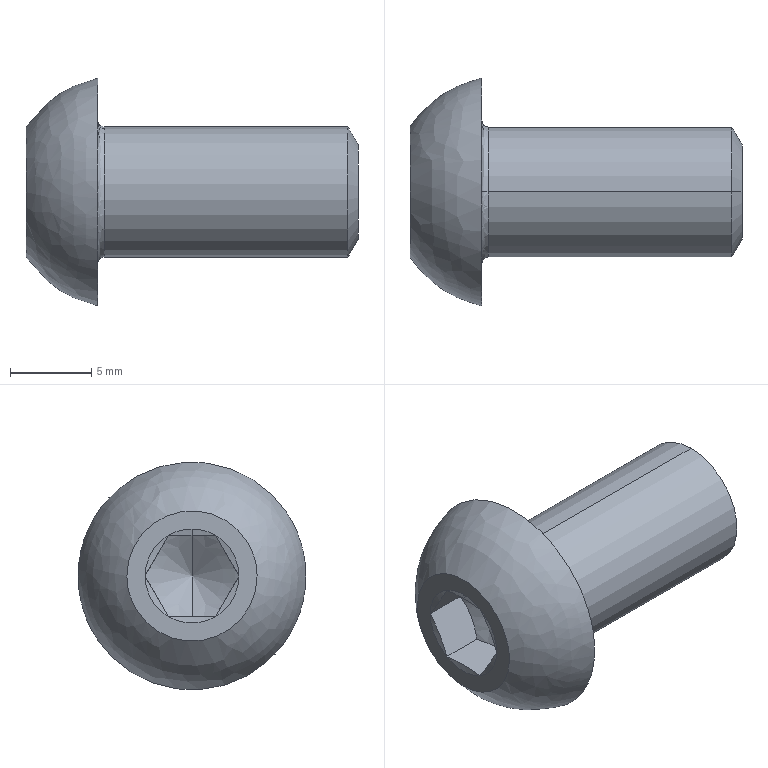Part | SolidWorks | features BaseBody 1 | 1 solid | 25 faces | box 20.4 x 14 x 14 mm | volume 1220 mm3 | cone 11 | plane 9 | spline 3 | cylinder 2 | commonest cylinder face diameters 8 x2
STEP:
#1=CARTESIAN_POINT('',(-15.6,0.,-4.));
#2=VERTEX_POINT('',#1);
#3=CARTESIAN_POINT('',(-15.6,0.,4.));
#4=VERTEX_POINT('',#3);
#5=CARTESIAN_POINT('',(-15.6,0.,0.));
#6=DIRECTION('',(1.,0.,0.));
#7=DIRECTION('',(0.,0.,1.));
#8=AXIS2_PLACEMENT_3D('',#5,#6,#7);
#9=CIRCLE('',#8,4.);
#10=EDGE_CURVE('',#2,#4,#9,.T.);
#11=ORIENTED_EDGE('',*,*,#10,.F.);
#12=CARTESIAN_POINT('',(-16.,0.,-4.4));
#13=VERTEX_POINT('',#12);
#14=CARTESIAN_POINT('',(-15.6,0.,-4.4));
#15=DIRECTION('',(0.,-1.,0.));
#16=DIRECTION('',(0.,0.,-1.));
#17=AXIS2_PLACEMENT_3D('',#14,#15,#16);
#18=CIRCLE('',#17,0.4);
#19=EDGE_CURVE('',#2,#13,#18,.T.);
#20=ORIENTED_EDGE('',*,*,#19,.T.);
#21=CARTESIAN_POINT('',(-16.,0.,4.4));
#22=VERTEX_POINT('',#21);
#23=CARTESIAN_POINT('',(-16.,0.,4.4));
#24=CARTESIAN_POINT('',(-16.,0.2798,4.4));
#25=CARTESIAN_POINT('',(-16.,0.6922,4.361));
#26=CARTESIAN_POINT('',(-16.,1.16,4.249));
#27=CARTESIAN_POINT('',(-16.,1.391,4.176));
#28=CARTESIAN_POINT('',(-16.,1.506,4.135));
#29=CARTESIAN_POINT('',(-16.,1.555,4.116));
#30=CARTESIAN_POINT('',(-16.,1.587,4.104));
#31=CARTESIAN_POINT('',(-16.,1.602,4.098));
#32=CARTESIAN_POINT('',(-16.,1.758,4.036));
#33=CARTESIAN_POINT('',(-16.,1.96,3.944));
#34=CARTESIAN_POINT('',(-16.,2.155,3.837));
#35=CARTESIAN_POINT('',(-16.,2.283,3.762));
#36=CARTESIAN_POINT('',(-16.,2.344,3.724));
#37=CARTESIAN_POINT('',(-16.,2.662,3.516));
#38=CARTESIAN_POINT('',(-16.,2.896,3.326));
#39=CARTESIAN_POINT('',(-16.,3.219,3.004));
#40=CARTESIAN_POINT('',(-16.,3.371,2.835));
#41=CARTESIAN_POINT('',(-16.,3.509,2.656));
#42=CARTESIAN_POINT('',(-16.,3.598,2.533));
#43=CARTESIAN_POINT('',(-16.,3.642,2.47));
#44=CARTESIAN_POINT('',(-16.,3.764,2.283));
#45=CARTESIAN_POINT('',(-16.,3.876,2.091));
#46=CARTESIAN_POINT('',(-16.,3.99,1.858));
#47=CARTESIAN_POINT('',(-16.,4.034,1.757));
#48=CARTESIAN_POINT('',(-16.,4.063,1.688));
#49=CARTESIAN_POINT('',(-16.,4.078,1.652));
#50=CARTESIAN_POINT('',(-16.,4.297,1.099));
#51=CARTESIAN_POINT('',(-16.,4.4,0.5599));
#52=CARTESIAN_POINT('',(-16.,4.4,-0.2799));
#53=CARTESIAN_POINT('',(-16.,4.361,-0.6923));
#54=CARTESIAN_POINT('',(-16.,4.249,-1.16));
#55=CARTESIAN_POINT('',(-16.,4.176,-1.391));
#56=CARTESIAN_POINT('',(-16.,4.135,-1.506));
#57=CARTESIAN_POINT('',(-16.,4.116,-1.555));
#58=CARTESIAN_POINT('',(-16.,4.104,-1.587));
#59=CARTESIAN_POINT('',(-16.,4.098,-1.602));
#60=CARTESIAN_POINT('',(-16.,4.036,-1.758));
#61=CARTESIAN_POINT('',(-16.,3.944,-1.96));
#62=CARTESIAN_POINT('',(-16.,3.837,-2.155));
#63=CARTESIAN_POINT('',(-16.,3.762,-2.283));
#64=CARTESIAN_POINT('',(-16.,3.724,-2.344));
#65=CARTESIAN_POINT('',(-16.,3.516,-2.662));
#66=CARTESIAN_POINT('',(-16.,3.326,-2.896));
#67=CARTESIAN_POINT('',(-16.,3.004,-3.219));
#68=CARTESIAN_POINT('',(-16.,2.835,-3.371));
#69=CARTESIAN_POINT('',(-16.,2.656,-3.509));
#70=CARTESIAN_POINT('',(-16.,2.533,-3.598));
#71=CARTESIAN_POINT('',(-16.,2.47,-3.642));
#72=CARTESIAN_POINT('',(-16.,2.283,-3.764));
#73=CARTESIAN_POINT('',(-16.,2.091,-3.876));
#74=CARTESIAN_POINT('',(-16.,1.858,-3.99));
#75=CARTESIAN_POINT('',(-16.,1.757,-4.034));
#76=CARTESIAN_POINT('',(-16.,1.688,-4.063));
#77=CARTESIAN_POINT('',(-16.,1.652,-4.078));
#78=CARTESIAN_POINT('',(-16.,1.099,-4.297));
#79=CARTESIAN_POINT('',(-16.,0.5593,-4.4));
#80=CARTESIAN_POINT('',(-16.,0.,-4.4));
#81=B_SPLINE_CURVE_WITH_KNOTS('',3,(#23,#24,#25,#26,#27,#28,#29,#30,#31,#32,#33,#34,#35,#36,#37,#38,#39,#40,#41,#42,#43,#44,#45,#46,#47,#48,#49,#50,#51,#52,#53,#54,#55,#56,#57,#58,#59,#60,#61,#62,#63,#64,#65,#66,#67,#68,#69,#70,#71,#72,#73,#74,#75,#76,#77,#78,#79,#80),.UNSPECIFIED.,.F.,.F.,(4,1,1,1,1,2,2,1,2,2,2,1,2,2,1,1,2,2,2,1,1,1,1,2,2,1,2,2,2,1,2,2,1,1,2,2,4),(0.,0.0625,0.09375,0.1094,0.1172,0.1211,0.125,0.1562,0.1719,0.1875,0.25,0.2812,0.2969,0.3125,0.3437,0.3594,0.3672,0.375,0.5,0.5625,0.5937,0.6094,0.6172,0.6211,0.625,0.6562,0.6719,0.6875,0.75,0.7812,0.7969,0.8125,0.8437,0.8594,0.8672,0.875,1.),.UNSPECIFIED.);
#82=EDGE_CURVE('',#22,#13,#81,.T.);
#83=ORIENTED_EDGE('',*,*,#82,.F.);
#84=CARTESIAN_POINT('',(-15.6,0.,4.4));
#85=DIRECTION('',(0.,1.,0.));
#86=DIRECTION('',(0.,0.,1.));
#87=AXIS2_PLACEMENT_3D('',#84,#85,#86);
#88=CIRCLE('',#87,0.4);
#89=EDGE_CURVE('',#4,#22,#88,.T.);
#90=ORIENTED_EDGE('',*,*,#89,.F.);
#91=EDGE_LOOP('',(#11,#20,#83,#90));
#92=FACE_OUTER_BOUND('',#91,.T.);
#93=CARTESIAN_POINT('',(-15.6,0.,4.));
#94=CARTESIAN_POINT('',(-15.6,8.,4.));
#95=CARTESIAN_POINT('',(-15.6,8.,-4.));
#96=CARTESIAN_POINT('',(-15.6,0.,-4.));
#97=CARTESIAN_POINT('',(-15.834,0.,4.));
#98=CARTESIAN_POINT('',(-15.834,8.,4.));
#99=CARTESIAN_POINT('',(-15.834,8.,-4.));
#100=CARTESIAN_POINT('',(-15.834,0.,-4.));
#101=CARTESIAN_POINT('',(-16.,0.,4.166));
#102=CARTESIAN_POINT('',(-16.,8.331,4.166));
#103=CARTESIAN_POINT('',(-16.,8.331,-4.166));
#104=CARTESIAN_POINT('',(-16.,0.,-4.166));
#105=CARTESIAN_POINT('',(-16.,0.,4.4));
#106=CARTESIAN_POINT('',(-16.,8.8,4.4));
#107=CARTESIAN_POINT('',(-16.,8.8,-4.4));
#108=CARTESIAN_POINT('',(-16.,0.,-4.4));
#109=(BOUNDED_SURFACE()B_SPLINE_SURFACE(3,3,((#93,#94,#95,#96),(#97,#98,#99,#100),(#101,#102,#103,#104),(#105,#106,#107,#108)),.UNSPECIFIED.,.F.,.F.,.F.)B_SPLINE_SURFACE_WITH_KNOTS((4,4),(4,4),(0.,1.),(0.,1.),.UNSPECIFIED.)GEOMETRIC_REPRESENTATION_ITEM()RATIONAL_B_SPLINE_SURFACE(((1.,0.3333,0.3333,1.),(0.8047,0.2682,0.2682,0.8047),(0.8047,0.2682,0.2682,0.8047),(1.,0.3333,0.3333,1.)))REPRESENTATION_ITEM('')SURFACE());
#110=ADVANCED_FACE('',(#92),#109,.F.);
#111=CARTESIAN_POINT('',(-0.625,0.,4.));
#112=VERTEX_POINT('',#111);
#113=CARTESIAN_POINT('',(-0.625,0.,-4.));
#114=VERTEX_POINT('',#113);
#115=CARTESIAN_POINT('',(-0.625,0.,0.));
#116=DIRECTION('',(-1.,0.,0.));
#117=DIRECTION('',(0.,0.,1.));
#118=AXIS2_PLACEMENT_3D('',#115,#116,#117);
#119=CIRCLE('',#118,4.);
#120=EDGE_CURVE('',#112,#114,#119,.T.);
#121=ORIENTED_EDGE('',*,*,#120,.T.);
#122=CARTESIAN_POINT('',(-20.4,0.,-4.));
#123=DIRECTION('',(-1.,0.,0.));
#124=VECTOR('',#123,1000.);
#125=LINE('',#122,#124);
#126=EDGE_CURVE('',#114,#2,#125,.T.);
#127=ORIENTED_EDGE('',*,*,#126,.T.);
#128=ORIENTED_EDGE('',*,*,#10,.T.);
#129=CARTESIAN_POINT('',(-20.4,0.,4.));
#130=DIRECTION('',(-1.,0.,0.));
#131=VECTOR('',#130,1000.);
#132=LINE('',#129,#131);
#133=EDGE_CURVE('',#112,#4,#132,.T.);
#134=ORIENTED_EDGE('',*,*,#133,.F.);
#135=EDGE_LOOP('',(#121,#127,#128,#134));
#136=FACE_OUTER_BOUND('',#135,.T.);
#137=CARTESIAN_POINT('',(-20.4,0.,0.));
#138=DIRECTION('',(-1.,0.,0.));
#139=DIRECTION('',(0.,0.,1.));
#140=AXIS2_PLACEMENT_3D('',#137,#138,#139);
#141=CYLINDRICAL_SURFACE('',#140,4.);
#142=ADVANCED_FACE('',(#136),#141,.T.);
#143=CARTESIAN_POINT('',(0.,0.,2.917));
#144=VERTEX_POINT('',#143);
#145=CARTESIAN_POINT('',(0.,0.,-2.917));
#146=VERTEX_POINT('',#145);
#147=CARTESIAN_POINT('',(0.,0.,0.));
#148=DIRECTION('',(-1.,0.,0.));
#149=DIRECTION('',(0.,0.,1.));
#150=AXIS2_PLACEMENT_3D('',#147,#148,#149);
#151=CIRCLE('',#150,2.917);
#152=EDGE_CURVE('',#144,#146,#151,.T.);
#153=ORIENTED_EDGE('',*,*,#152,.T.);
#154=CARTESIAN_POINT('',(-0.625,0.,-4.));
#155=DIRECTION('',(-0.5,0.,-0.866));
#156=VECTOR('',#155,1000.);
#157=LINE('',#154,#156);
#158=EDGE_CURVE('',#146,#114,#157,.T.);
#159=ORIENTED_EDGE('',*,*,#158,.T.);
#160=ORIENTED_EDGE('',*,*,#120,.F.);
#161=CARTESIAN_POINT('',(-0.625,0.,4.));
#162=DIRECTION('',(-0.5,0.,0.866));
#163=VECTOR('',#162,1000.);
#164=LINE('',#161,#163);
#165=EDGE_CURVE('',#144,#112,#164,.T.);
#166=ORIENTED_EDGE('',*,*,#165,.F.);
#167=EDGE_LOOP('',(#153,#159,#160,#166));
#168=FACE_OUTER_BOUND('',#167,.T.);
#169=CARTESIAN_POINT('',(-0.625,0.,0.));
#170=DIRECTION('',(-1.,0.,0.));
#171=DIRECTION('',(0.,0.,1.));
#172=AXIS2_PLACEMENT_3D('',#169,#170,#171);
#173=CONICAL_SURFACE('',#172,4.,1.047);
#174=ADVANCED_FACE('',(#168),#173,.T.);
#175=CARTESIAN_POINT('',(-20.4,1.443,2.5));
#176=VERTEX_POINT('',#175);
#177=CARTESIAN_POINT('',(-20.304,0.,2.5));
#178=VERTEX_POINT('',#177);
#179=CARTESIAN_POINT('',(-20.4,1.443,2.5));
#180=CARTESIAN_POINT('',(-20.34,0.9641,2.5));
#181=CARTESIAN_POINT('',(-20.304,0.4833,2.5));
#182=CARTESIAN_POINT('',(-20.304,0.,2.5));
#183=B_SPLINE_CURVE_WITH_KNOTS('',3,(#179,#180,#181,#182),.UNSPECIFIED.,.F.,.F.,(4,4),(0.,0.001447),.UNSPECIFIED.);
#184=EDGE_CURVE('',#176,#178,#183,.T.);
#185=ORIENTED_EDGE('',*,*,#184,.T.);
#186=CARTESIAN_POINT('',(-20.4,0.,2.887));
#187=VERTEX_POINT('',#186);
#188=CARTESIAN_POINT('',(-20.4,0.,2.887));
#189=DIRECTION('',(-0.242,0.,0.9703));
#190=VECTOR('',#189,1000.);
#191=LINE('',#188,#190);
#192=EDGE_CURVE('',#178,#187,#191,.T.);
#193=ORIENTED_EDGE('',*,*,#192,.T.);
#194=CARTESIAN_POINT('',(-20.4,0.,0.));
#195=DIRECTION('',(-1.,0.,0.));
#196=DIRECTION('',(0.,0.,1.));
#197=AXIS2_PLACEMENT_3D('',#194,#195,#196);
#198=CIRCLE('',#197,2.887);
#199=EDGE_CURVE('',#187,#176,#198,.T.);
#200=ORIENTED_EDGE('',*,*,#199,.T.);
#201=EDGE_LOOP('',(#185,#193,#200));
#202=FACE_OUTER_BOUND('',#201,.T.);
#203=CARTESIAN_POINT('',(-20.4,0.,0.));
#204=DIRECTION('',(-1.,0.,0.));
#205=DIRECTION('',(0.,0.,1.));
#206=AXIS2_PLACEMENT_3D('',#203,#204,#205);
#207=CONICAL_SURFACE('',#206,2.887,1.326);
#208=ADVANCED_FACE('',(#202),#207,.F.);
#209=CARTESIAN_POINT('',(-16.,0.,0.));
#210=VERTEX_POINT('',#209);
#211=CARTESIAN_POINT('',(-17.559,0.,2.5));
#212=VERTEX_POINT('',#211);
#213=CARTESIAN_POINT('',(-17.811,0.,2.904));
#214=DIRECTION('',(-0.5291,0.,0.8486));
#215=VECTOR('',#214,1000.);
#216=LINE('',#213,#215);
#217=EDGE_CURVE('',#210,#212,#216,.T.);
#218=ORIENTED_EDGE('',*,*,#217,.F.);
#219=CARTESIAN_POINT('',(-17.559,0.,-2.5));
#220=VERTEX_POINT('',#219);
#221=CARTESIAN_POINT('',(-17.811,0.,-2.904));
#222=DIRECTION('',(-0.5291,0.,-0.8486));
#223=VECTOR('',#222,1000.);
#224=LINE('',#221,#223);
#225=EDGE_CURVE('',#210,#220,#224,.T.);
#226=ORIENTED_EDGE('',*,*,#225,.T.);
#227=CARTESIAN_POINT('',(-17.8,-1.443,-2.5));
#228=VERTEX_POINT('',#227);
#229=CARTESIAN_POINT('',(-17.559,0.,-2.5));
#230=CARTESIAN_POINT('',(-17.559,-0.4946,-2.5));
#231=CARTESIAN_POINT('',(-17.653,-0.9733,-2.5));
#232=CARTESIAN_POINT('',(-17.8,-1.443,-2.5));
#233=B_SPLINE_CURVE_WITH_KNOTS('',3,(#229,#230,#231,#232),.UNSPECIFIED.,.F.,.F.,(4,4),(0.,0.001463),.UNSPECIFIED.);
#234=EDGE_CURVE('',#220,#228,#233,.T.);
#235=ORIENTED_EDGE('',*,*,#234,.T.);
#236=CARTESIAN_POINT('',(-17.8,-2.887,0.));
#237=VERTEX_POINT('',#236);
#238=CARTESIAN_POINT('',(-17.8,-1.443,-2.5));
#239=CARTESIAN_POINT('',(-17.654,-1.678,-2.093));
#240=CARTESIAN_POINT('',(-17.559,-1.917,-1.679));
#241=CARTESIAN_POINT('',(-17.559,-2.286,-1.04));
#242=CARTESIAN_POINT('',(-17.582,-2.409,-0.8268));
#243=CARTESIAN_POINT('',(-17.666,-2.65,-0.4095));
#244=CARTESIAN_POINT('',(-17.727,-2.769,-0.2038));
#245=CARTESIAN_POINT('',(-17.8,-2.887,0.));
#246=B_SPLINE_CURVE_WITH_KNOTS('',3,(#238,#239,#240,#241,#242,#243,#244,#245),.UNSPECIFIED.,.F.,.F.,(4,2,2,4),(0.,0.00146,0.002189,0.002919),.UNSPECIFIED.);
#247=EDGE_CURVE('',#228,#237,#246,.T.);
#248=ORIENTED_EDGE('',*,*,#247,.T.);
#249=CARTESIAN_POINT('',(-17.8,-1.443,2.5));
#250=VERTEX_POINT('',#249);
#251=CARTESIAN_POINT('',(-17.8,-2.887,0.));
#252=CARTESIAN_POINT('',(-17.654,-2.652,0.4068));
#253=CARTESIAN_POINT('',(-17.559,-2.413,0.8206));
#254=CARTESIAN_POINT('',(-17.559,-2.044,1.46));
#255=CARTESIAN_POINT('',(-17.582,-1.921,1.673));
#256=CARTESIAN_POINT('',(-17.666,-1.68,2.09));
#257=CARTESIAN_POINT('',(-17.727,-1.561,2.296));
#258=CARTESIAN_POINT('',(-17.8,-1.443,2.5));
#259=B_SPLINE_CURVE_WITH_KNOTS('',3,(#251,#252,#253,#254,#255,#256,#257,#258),.UNSPECIFIED.,.F.,.F.,(4,2,2,4),(0.,0.00146,0.002189,0.002919),.UNSPECIFIED.);
#260=EDGE_CURVE('',#237,#250,#259,.T.);
#261=ORIENTED_EDGE('',*,*,#260,.T.);
#262=CARTESIAN_POINT('',(-17.559,0.,2.5));
#263=CARTESIAN_POINT('',(-17.559,-0.4946,2.5));
#264=CARTESIAN_POINT('',(-17.653,-0.9733,2.5));
#265=CARTESIAN_POINT('',(-17.8,-1.443,2.5));
#266=B_SPLINE_CURVE_WITH_KNOTS('',3,(#262,#263,#264,#265),.UNSPECIFIED.,.F.,.F.,(4,4),(0.,0.001463),.UNSPECIFIED.);
#267=EDGE_CURVE('',#212,#250,#266,.T.);
#268=ORIENTED_EDGE('',*,*,#267,.F.);
#269=EDGE_LOOP('',(#218,#226,#235,#248,#261,#268));
#270=FACE_OUTER_BOUND('',#269,.T.);
#271=CARTESIAN_POINT('',(-17.811,0.,0.));
#272=DIRECTION('',(-1.,0.,0.));
#273=DIRECTION('',(0.,0.,1.));
#274=AXIS2_PLACEMENT_3D('',#271,#272,#273);
#275=CONICAL_SURFACE('',#274,2.904,1.013);
#276=ADVANCED_FACE('',(#270),#275,.F.);
#277=ORIENTED_EDGE('',*,*,#126,.F.);
#278=CARTESIAN_POINT('',(-0.625,0.,0.));
#279=DIRECTION('',(-1.,0.,0.));
#280=DIRECTION('',(0.,0.,1.));
#281=AXIS2_PLACEMENT_3D('',#278,#279,#280);
#282=CIRCLE('',#281,4.);
#283=EDGE_CURVE('',#114,#112,#282,.T.);
#284=ORIENTED_EDGE('',*,*,#283,.T.);
#285=ORIENTED_EDGE('',*,*,#133,.T.);
#286=CARTESIAN_POINT('',(-15.6,0.,0.));
#287=DIRECTION('',(1.,0.,0.));
#288=DIRECTION('',(0.,0.,1.));
#289=AXIS2_PLACEMENT_3D('',#286,#287,#288);
#290=CIRCLE('',#289,4.);
#291=EDGE_CURVE('',#4,#2,#290,.T.);
#292=ORIENTED_EDGE('',*,*,#291,.T.);
#293=EDGE_LOOP('',(#277,#284,#285,#292));
#294=FACE_OUTER_BOUND('',#293,.T.);
#295=CARTESIAN_POINT('',(-20.4,0.,0.));
#296=DIRECTION('',(-1.,0.,0.));
#297=DIRECTION('',(0.,0.,1.));
#298=AXIS2_PLACEMENT_3D('',#295,#296,#297);
#299=CYLINDRICAL_SURFACE('',#298,4.);
#300=ADVANCED_FACE('',(#294),#299,.T.);
#301=ORIENTED_EDGE('',*,*,#19,.F.);
#302=ORIENTED_EDGE('',*,*,#291,.F.);
#303=ORIENTED_EDGE('',*,*,#89,.T.);
#304=CARTESIAN_POINT('',(-16.,0.,-4.4));
#305=CARTESIAN_POINT('',(-16.,-0.2798,-4.4));
#306=CARTESIAN_POINT('',(-16.,-0.6922,-4.361));
#307=CARTESIAN_POINT('',(-16.,-1.16,-4.249));
#308=CARTESIAN_POINT('',(-16.,-1.391,-4.176));
#309=CARTESIAN_POINT('',(-16.,-1.506,-4.135));
#310=CARTESIAN_POINT('',(-16.,-1.555,-4.116));
#311=CARTESIAN_POINT('',(-16.,-1.587,-4.104));
#312=CARTESIAN_POINT('',(-16.,-1.602,-4.098));
#313=CARTESIAN_POINT('',(-16.,-1.758,-4.036));
#314=CARTESIAN_POINT('',(-16.,-1.96,-3.944));
#315=CARTESIAN_POINT('',(-16.,-2.155,-3.837));
#316=CARTESIAN_POINT('',(-16.,-2.283,-3.762));
#317=CARTESIAN_POINT('',(-16.,-2.344,-3.724));
#318=CARTESIAN_POINT('',(-16.,-2.662,-3.516));
#319=CARTESIAN_POINT('',(-16.,-2.896,-3.326));
#320=CARTESIAN_POINT('',(-16.,-3.219,-3.004));
#321=CARTESIAN_POINT('',(-16.,-3.371,-2.835));
#322=CARTESIAN_POINT('',(-16.,-3.509,-2.656));
#323=CARTESIAN_POINT('',(-16.,-3.598,-2.533));
#324=CARTESIAN_POINT('',(-16.,-3.642,-2.47));
#325=CARTESIAN_POINT('',(-16.,-3.764,-2.283));
#326=CARTESIAN_POINT('',(-16.,-3.876,-2.091));
#327=CARTESIAN_POINT('',(-16.,-3.99,-1.858));
#328=CARTESIAN_POINT('',(-16.,-4.034,-1.757));
#329=CARTESIAN_POINT('',(-16.,-4.063,-1.688));
#330=CARTESIAN_POINT('',(-16.,-4.078,-1.652));
#331=CARTESIAN_POINT('',(-16.,-4.297,-1.099));
#332=CARTESIAN_POINT('',(-16.,-4.4,-0.5599));
#333=CARTESIAN_POINT('',(-16.,-4.4,0.2799));
#334=CARTESIAN_POINT('',(-16.,-4.361,0.6923));
#335=CARTESIAN_POINT('',(-16.,-4.249,1.16));
#336=CARTESIAN_POINT('',(-16.,-4.176,1.391));
#337=CARTESIAN_POINT('',(-16.,-4.135,1.506));
#338=CARTESIAN_POINT('',(-16.,-4.116,1.555));
#339=CARTESIAN_POINT('',(-16.,-4.104,1.587));
#340=CARTESIAN_POINT('',(-16.,-4.098,1.602));
#341=CARTESIAN_POINT('',(-16.,-4.036,1.758));
#342=CARTESIAN_POINT('',(-16.,-3.944,1.96));
#343=CARTESIAN_POINT('',(-16.,-3.837,2.155));
#344=CARTESIAN_POINT('',(-16.,-3.762,2.283));
#345=CARTESIAN_POINT('',(-16.,-3.724,2.344));
#346=CARTESIAN_POINT('',(-16.,-3.516,2.662));
#347=CARTESIAN_POINT('',(-16.,-3.326,2.896));
#348=CARTESIAN_POINT('',(-16.,-3.004,3.219));
#349=CARTESIAN_POINT('',(-16.,-2.835,3.371));
#350=CARTESIAN_POINT('',(-16.,-2.656,3.509));
#351=CARTESIAN_POINT('',(-16.,-2.533,3.598));
#352=CARTESIAN_POINT('',(-16.,-2.47,3.642));
#353=CARTESIAN_POINT('',(-16.,-2.283,3.764));
#354=CARTESIAN_POINT('',(-16.,-2.091,3.876));
#355=CARTESIAN_POINT('',(-16.,-1.858,3.99));
#356=CARTESIAN_POINT('',(-16.,-1.757,4.034));
#357=CARTESIAN_POINT('',(-16.,-1.688,4.063));
#358=CARTESIAN_POINT('',(-16.,-1.652,4.078));
#359=CARTESIAN_POINT('',(-16.,-1.099,4.297));
#360=CARTESIAN_POINT('',(-16.,-0.5593,4.4));
#361=CARTESIAN_POINT('',(-16.,0.,4.4));
#362=B_SPLINE_CURVE_WITH_KNOTS('',3,(#304,#305,#306,#307,#308,#309,#310,#311,#312,#313,#314,#315,#316,#317,#318,#319,#320,#321,#322,#323,#324,#325,#326,#327,#328,#329,#330,#331,#332,#333,#334,#335,#336,#337,#338,#339,#340,#341,#342,#343,#344,#345,#346,#347,#348,#349,#350,#351,#352,#353,#354,#355,#356,#357,#358,#359,#360,#361),.UNSPECIFIED.,.F.,.F.,(4,1,1,1,1,2,2,1,2,2,2,1,2,2,1,1,2,2,2,1,1,1,1,2,2,1,2,2,2,1,2,2,1,1,2,2,4),(0.,0.0625,0.09375,0.1094,0.1172,0.1211,0.125,0.1563,0.1719,0.1875,0.25,0.2813,0.2969,0.3125,0.3438,0.3594,0.3672,0.375,0.5,0.5625,0.5938,0.6094,0.6172,0.6211,0.625,0.6563,0.6719,0.6875,0.75,0.7813,0.7969,0.8125,0.8438,0.8594,0.8672,0.875,1.),.UNSPECIFIED.);
#363=EDGE_CURVE('',#13,#22,#362,.T.);
#364=ORIENTED_EDGE('',*,*,#363,.F.);
#365=EDGE_LOOP('',(#301,#302,#303,#364));
#366=FACE_OUTER_BOUND('',#365,.T.);
#367=CARTESIAN_POINT('',(-15.6,0.,-4.));
#368=CARTESIAN_POINT('',(-15.6,-8.,-4.));
#369=CARTESIAN_POINT('',(-15.6,-8.,4.));
#370=CARTESIAN_POINT('',(-15.6,0.,4.));
#371=CARTESIAN_POINT('',(-15.834,0.,-4.));
#372=CARTESIAN_POINT('',(-15.834,-8.,-4.));
#373=CARTESIAN_POINT('',(-15.834,-8.,4.));
#374=CARTESIAN_POINT('',(-15.834,0.,4.));
#375=CARTESIAN_POINT('',(-16.,0.,-4.166));
#376=CARTESIAN_POINT('',(-16.,-8.331,-4.166));
#377=CARTESIAN_POINT('',(-16.,-8.331,4.166));
#378=CARTESIAN_POINT('',(-16.,0.,4.166));
#379=CARTESIAN_POINT('',(-16.,0.,-4.4));
#380=CARTESIAN_POINT('',(-16.,-8.8,-4.4));
#381=CARTESIAN_POINT('',(-16.,-8.8,4.4));
#382=CARTESIAN_POINT('',(-16.,0.,4.4));
#383=(BOUNDED_SURFACE()B_SPLINE_SURFACE(3,3,((#367,#368,#369,#370),(#371,#372,#373,#374),(#375,#376,#377,#378),(#379,#380,#381,#382)),.UNSPECIFIED.,.F.,.F.,.F.)B_SPLINE_SURFACE_WITH_KNOTS((4,4),(4,4),(0.,1.),(0.,1.),.UNSPECIFIED.)GEOMETRIC_REPRESENTATION_ITEM()RATIONAL_B_SPLINE_SURFACE(((1.,0.3333,0.3333,1.),(0.8047,0.2682,0.2682,0.8047),(0.8047,0.2682,0.2682,0.8047),(1.,0.3333,0.3333,1.)))REPRESENTATION_ITEM('')SURFACE());
#384=ADVANCED_FACE('',(#366),#383,.F.);
#385=ORIENTED_EDGE('',*,*,#158,.F.);
#386=CARTESIAN_POINT('',(0.,0.,0.));
#387=DIRECTION('',(-1.,0.,0.));
#388=DIRECTION('',(0.,0.,1.));
#389=AXIS2_PLACEMENT_3D('',#386,#387,#388);
#390=CIRCLE('',#389,2.917);
#391=EDGE_CURVE('',#146,#144,#390,.T.);
#392=ORIENTED_EDGE('',*,*,#391,.T.);
#393=ORIENTED_EDGE('',*,*,#165,.T.);
#394=ORIENTED_EDGE('',*,*,#283,.F.);
#395=EDGE_LOOP('',(#385,#392,#393,#394));
#396=FACE_OUTER_BOUND('',#395,.T.);
#397=CARTESIAN_POINT('',(-0.625,0.,0.));
#398=DIRECTION('',(-1.,0.,0.));
#399=DIRECTION('',(0.,0.,1.));
#400=AXIS2_PLACEMENT_3D('',#397,#398,#399);
#401=CONICAL_SURFACE('',#400,4.,1.047);
#402=ADVANCED_FACE('',(#396),#401,.T.);
#403=ORIENTED_EDGE('',*,*,#363,.T.);
#404=ORIENTED_EDGE('',*,*,#82,.T.);
#405=EDGE_LOOP('',(#403,#404));
#406=FACE_BOUND('',#405,.T.);
#407=CARTESIAN_POINT('',(-16.,7.,0.));
#408=VERTEX_POINT('',#407);
#409=CARTESIAN_POINT('',(-16.,-7.,0.));
#410=VERTEX_POINT('',#409);
#411=CARTESIAN_POINT('',(-16.,7.,0.));
#412=CARTESIAN_POINT('',(-16.,7.,-0.4622));
#413=CARTESIAN_POINT('',(-16.,6.955,-0.9197));
#414=CARTESIAN_POINT('',(-16.,6.774,-1.825));
#415=CARTESIAN_POINT('',(-16.,6.64,-2.263));
#416=CARTESIAN_POINT('',(-16.,6.378,-2.895));
#417=CARTESIAN_POINT('',(-16.,6.28,-3.101));
#418=CARTESIAN_POINT('',(-16.,6.063,-3.506));
#419=CARTESIAN_POINT('',(-16.,5.944,-3.704));
#420=CARTESIAN_POINT('',(-16.,5.561,-4.277));
#421=CARTESIAN_POINT('',(-16.,5.271,-4.629));
#422=CARTESIAN_POINT('',(-16.,4.625,-5.274));
#423=CARTESIAN_POINT('',(-16.,4.264,-5.57));
#424=CARTESIAN_POINT('',(-16.,3.505,-6.077));
#425=CARTESIAN_POINT('',(-16.,3.103,-6.292));
#426=CARTESIAN_POINT('',(-16.,2.466,-6.555));
#427=CARTESIAN_POINT('',(-16.,2.248,-6.633));
#428=CARTESIAN_POINT('',(-16.,1.809,-6.766));
#429=CARTESIAN_POINT('',(-16.,1.587,-6.821));
#430=CARTESIAN_POINT('',(-16.,0.917,-6.955));
#431=CARTESIAN_POINT('',(-16.,0.4599,-7.));
#432=CARTESIAN_POINT('',(-16.,-0.4622,-7.));
#433=CARTESIAN_POINT('',(-16.,-0.9163,-6.955));
#434=CARTESIAN_POINT('',(-16.,-1.587,-6.821));
#435=CARTESIAN_POINT('',(-16.,-1.809,-6.766));
#436=CARTESIAN_POINT('',(-16.,-2.25,-6.633));
#437=CARTESIAN_POINT('',(-16.,-2.468,-6.555));
#438=CARTESIAN_POINT('',(-16.,-3.102,-6.292));
#439=CARTESIAN_POINT('',(-16.,-3.504,-6.077));
#440=CARTESIAN_POINT('',(-16.,-4.075,-5.696));
#441=CARTESIAN_POINT('',(-16.,-4.261,-5.558));
#442=CARTESIAN_POINT('',(-16.,-4.617,-5.266));
#443=CARTESIAN_POINT('',(-16.,-4.787,-5.113));
#444=CARTESIAN_POINT('',(-16.,-5.271,-4.629));
#445=CARTESIAN_POINT('',(-16.,-5.561,-4.277));
#446=CARTESIAN_POINT('',(-16.,-6.073,-3.511));
#447=CARTESIAN_POINT('',(-16.,-6.29,-3.105));
#448=CARTESIAN_POINT('',(-16.,-6.552,-2.474));
#449=CARTESIAN_POINT('',(-16.,-6.629,-2.259));
#450=CARTESIAN_POINT('',(-16.,-6.763,-1.821));
#451=CARTESIAN_POINT('',(-16.,-6.819,-1.596));
#452=CARTESIAN_POINT('',(-16.,-6.955,-0.919));
#453=CARTESIAN_POINT('',(-16.,-7.,-0.4622));
#454=CARTESIAN_POINT('',(-16.,-7.,0.));
#455=B_SPLINE_CURVE_WITH_KNOTS('',3,(#411,#412,#413,#414,#415,#416,#417,#418,#419,#420,#421,#422,#423,#424,#425,#426,#427,#428,#429,#430,#431,#432,#433,#434,#435,#436,#437,#438,#439,#440,#441,#442,#443,#444,#445,#446,#447,#448,#449,#450,#451,#452,#453,#454),.UNSPECIFIED.,.F.,.F.,(4,2,2,2,2,2,2,2,2,2,2,2,2,2,2,2,2,2,2,2,2,4),(0.,0.001379,0.002758,0.003448,0.004138,0.005517,0.006896,0.008275,0.008965,0.009654,0.01103,0.01241,0.0131,0.01379,0.01517,0.01586,0.01655,0.01793,0.01931,0.02,0.02069,0.02207),.UNSPECIFIED.);
#456=EDGE_CURVE('',#408,#410,#455,.T.);
#457=ORIENTED_EDGE('',*,*,#456,.F.);
#458=CARTESIAN_POINT('',(-16.,-7.,0.));
#459=CARTESIAN_POINT('',(-16.,-7.,0.4622));
#460=CARTESIAN_POINT('',(-16.,-6.955,0.9197));
#461=CARTESIAN_POINT('',(-16.,-6.774,1.825));
#462=CARTESIAN_POINT('',(-16.,-6.64,2.263));
#463=CARTESIAN_POINT('',(-16.,-6.378,2.895));
#464=CARTESIAN_POINT('',(-16.,-6.28,3.101));
#465=CARTESIAN_POINT('',(-16.,-6.063,3.506));
#466=CARTESIAN_POINT('',(-16.,-5.944,3.704));
#467=CARTESIAN_POINT('',(-16.,-5.561,4.277));
#468=CARTESIAN_POINT('',(-16.,-5.271,4.629));
#469=CARTESIAN_POINT('',(-16.,-4.625,5.274));
#470=CARTESIAN_POINT('',(-16.,-4.264,5.57));
#471=CARTESIAN_POINT('',(-16.,-3.505,6.077));
#472=CARTESIAN_POINT('',(-16.,-3.103,6.292));
#473=CARTESIAN_POINT('',(-16.,-2.466,6.555));
#474=CARTESIAN_POINT('',(-16.,-2.248,6.633));
#475=CARTESIAN_POINT('',(-16.,-1.809,6.766));
#476=CARTESIAN_POINT('',(-16.,-1.587,6.821));
#477=CARTESIAN_POINT('',(-16.,-0.917,6.955));
#478=CARTESIAN_POINT('',(-16.,-0.4599,7.));
#479=CARTESIAN_POINT('',(-16.,0.4622,7.));
#480=CARTESIAN_POINT('',(-16.,0.9163,6.955));
#481=CARTESIAN_POINT('',(-16.,1.587,6.821));
#482=CARTESIAN_POINT('',(-16.,1.809,6.766));
#483=CARTESIAN_POINT('',(-16.,2.25,6.633));
#484=CARTESIAN_POINT('',(-16.,2.468,6.555));
#485=CARTESIAN_POINT('',(-16.,3.102,6.292));
#486=CARTESIAN_POINT('',(-16.,3.504,6.077));
#487=CARTESIAN_POINT('',(-16.,4.075,5.696));
#488=CARTESIAN_POINT('',(-16.,4.261,5.558));
#489=CARTESIAN_POINT('',(-16.,4.617,5.266));
#490=CARTESIAN_POINT('',(-16.,4.787,5.113));
#491=CARTESIAN_POINT('',(-16.,5.271,4.629));
#492=CARTESIAN_POINT('',(-16.,5.561,4.277));
#493=CARTESIAN_POINT('',(-16.,6.073,3.511));
#494=CARTESIAN_POINT('',(-16.,6.29,3.105));
#495=CARTESIAN_POINT('',(-16.,6.552,2.474));
#496=CARTESIAN_POINT('',(-16.,6.629,2.259));
#497=CARTESIAN_POINT('',(-16.,6.763,1.821));
#498=CARTESIAN_POINT('',(-16.,6.819,1.596));
#499=CARTESIAN_POINT('',(-16.,6.955,0.919));
#500=CARTESIAN_POINT('',(-16.,7.,0.4622));
#501=CARTESIAN_POINT('',(-16.,7.,0.));
#502=B_SPLINE_CURVE_WITH_KNOTS('',3,(#458,#459,#460,#461,#462,#463,#464,#465,#466,#467,#468,#469,#470,#471,#472,#473,#474,#475,#476,#477,#478,#479,#480,#481,#482,#483,#484,#485,#486,#487,#488,#489,#490,#491,#492,#493,#494,#495,#496,#497,#498,#499,#500,#501),.UNSPECIFIED.,.F.,.F.,(4,2,2,2,2,2,2,2,2,2,2,2,2,2,2,2,2,2,2,2,2,4),(0.02207,0.02345,0.02483,0.02552,0.0262,0.02758,0.02896,0.03034,0.03103,0.03172,0.0331,0.03448,0.03517,0.03586,0.03724,0.03793,0.03862,0.04,0.04138,0.04207,0.04276,0.04413),.UNSPECIFIED.);
#503=EDGE_CURVE('',#410,#408,#502,.T.);
#504=ORIENTED_EDGE('',*,*,#503,.F.);
#505=EDGE_LOOP('',(#457,#504));
#506=FACE_OUTER_BOUND('',#505,.T.);
#507=CARTESIAN_POINT('',(-16.,4.4,0.));
#508=DIRECTION('',(-1.,0.,0.));
#509=DIRECTION('',(0.,0.,1.));
#510=AXIS2_PLACEMENT_3D('',#507,#508,#509);
#511=PLANE('',#510);
#512=ADVANCED_FACE('',(#406,#506),#511,.F.);
#513=ORIENTED_EDGE('',*,*,#152,.F.);
#514=ORIENTED_EDGE('',*,*,#391,.F.);
#515=EDGE_LOOP('',(#513,#514));
#516=FACE_OUTER_BOUND('',#515,.T.);
#517=CARTESIAN_POINT('',(0.,4.,0.));
#518=DIRECTION('',(-1.,0.,0.));
#519=DIRECTION('',(0.,0.,1.));
#520=AXIS2_PLACEMENT_3D('',#517,#518,#519);
#521=PLANE('',#520);
#522=ADVANCED_FACE('',(#516),#521,.F.);
#523=CARTESIAN_POINT('',(-20.4,-4.,0.));
#524=VERTEX_POINT('',#523);
#525=CARTESIAN_POINT('',(-20.4,4.,0.));
#526=VERTEX_POINT('',#525);
#527=CARTESIAN_POINT('',(-20.4,-4.,0.));
#528=CARTESIAN_POINT('',(-20.4,-4.,-0.2642));
#529=CARTESIAN_POINT('',(-20.4,-3.974,-0.5241));
#530=CARTESIAN_POINT('',(-20.4,-3.872,-1.035));
#531=CARTESIAN_POINT('',(-20.4,-3.796,-1.289));
#532=CARTESIAN_POINT('',(-20.4,-3.595,-1.774));
#533=CARTESIAN_POINT('',(-20.4,-3.472,-2.003));
#534=CARTESIAN_POINT('',(-20.4,-3.182,-2.438));
#535=CARTESIAN_POINT('',(-20.4,-3.013,-2.644));
#536=CARTESIAN_POINT('',(-20.4,-2.644,-3.013));
#537=CARTESIAN_POINT('',(-20.4,-2.443,-3.179));
#538=CARTESIAN_POINT('',(-20.4,-2.005,-3.471));
#539=CARTESIAN_POINT('',(-20.4,-1.773,-3.595));
#540=CARTESIAN_POINT('',(-20.4,-1.291,-3.795));
#541=CARTESIAN_POINT('',(-20.4,-1.039,-3.872));
#542=CARTESIAN_POINT('',(-20.4,-0.523,-3.974));
#543=CARTESIAN_POINT('',(-20.4,-0.2635,-4.));
#544=CARTESIAN_POINT('',(-20.4,0.2581,-4.));
#545=CARTESIAN_POINT('',(-20.4,0.5231,-3.974));
#546=CARTESIAN_POINT('',(-20.4,1.036,-3.872));
#547=CARTESIAN_POINT('',(-20.4,1.285,-3.797));
#548=CARTESIAN_POINT('',(-20.4,1.77,-3.597));
#549=CARTESIAN_POINT('',(-20.4,2.004,-3.472));
#550=CARTESIAN_POINT('',(-20.4,2.437,-3.182));
#551=CARTESIAN_POINT('',(-20.4,2.64,-3.017));
#552=CARTESIAN_POINT('',(-20.4,3.013,-2.644));
#553=CARTESIAN_POINT('',(-20.4,3.179,-2.442));
#554=CARTESIAN_POINT('',(-20.4,3.469,-2.009));
#555=CARTESIAN_POINT('',(-20.4,3.594,-1.775));
#556=CARTESIAN_POINT('',(-20.4,3.795,-1.29));
#557=CARTESIAN_POINT('',(-20.4,3.871,-1.041));
#558=CARTESIAN_POINT('',(-20.4,3.974,-0.5286));
#559=CARTESIAN_POINT('',(-20.4,4.,-0.2642));
#560=CARTESIAN_POINT('',(-20.4,4.,0.));
#561=B_SPLINE_CURVE_WITH_KNOTS('',3,(#527,#528,#529,#530,#531,#532,#533,#534,#535,#536,#537,#538,#539,#540,#541,#542,#543,#544,#545,#546,#547,#548,#549,#550,#551,#552,#553,#554,#555,#556,#557,#558,#559,#560),.UNSPECIFIED.,.F.,.F.,(4,2,2,2,2,2,2,2,2,2,2,2,2,2,2,2,4),(0.,0.0007815,0.001563,0.002344,0.003126,0.003907,0.004689,0.00547,0.006252,0.007033,0.007815,0.008596,0.009377,0.01016,0.01094,0.01172,0.0125),.UNSPECIFIED.);
#562=EDGE_CURVE('',#524,#526,#561,.T.);
#563=ORIENTED_EDGE('',*,*,#562,.T.);
#564=CARTESIAN_POINT('',(-20.4,4.,0.));
#565=CARTESIAN_POINT('',(-20.4,4.,0.2642));
#566=CARTESIAN_POINT('',(-20.4,3.974,0.5241));
#567=CARTESIAN_POINT('',(-20.4,3.872,1.035));
#568=CARTESIAN_POINT('',(-20.4,3.796,1.289));
#569=CARTESIAN_POINT('',(-20.4,3.595,1.774));
#570=CARTESIAN_POINT('',(-20.4,3.472,2.003));
#571=CARTESIAN_POINT('',(-20.4,3.182,2.438));
#572=CARTESIAN_POINT('',(-20.4,3.013,2.644));
#573=CARTESIAN_POINT('',(-20.4,2.644,3.013));
#574=CARTESIAN_POINT('',(-20.4,2.443,3.179));
#575=CARTESIAN_POINT('',(-20.4,2.005,3.471));
#576=CARTESIAN_POINT('',(-20.4,1.773,3.595));
#577=CARTESIAN_POINT('',(-20.4,1.291,3.795));
#578=CARTESIAN_POINT('',(-20.4,1.039,3.872));
#579=CARTESIAN_POINT('',(-20.4,0.523,3.974));
#580=CARTESIAN_POINT('',(-20.4,0.2635,4.));
#581=CARTESIAN_POINT('',(-20.4,-0.2581,4.));
#582=CARTESIAN_POINT('',(-20.4,-0.5231,3.974));
#583=CARTESIAN_POINT('',(-20.4,-1.036,3.872));
#584=CARTESIAN_POINT('',(-20.4,-1.285,3.797));
#585=CARTESIAN_POINT('',(-20.4,-1.77,3.597));
#586=CARTESIAN_POINT('',(-20.4,-2.004,3.472));
#587=CARTESIAN_POINT('',(-20.4,-2.437,3.182));
#588=CARTESIAN_POINT('',(-20.4,-2.64,3.017));
#589=CARTESIAN_POINT('',(-20.4,-3.013,2.644));
#590=CARTESIAN_POINT('',(-20.4,-3.179,2.442));
#591=CARTESIAN_POINT('',(-20.4,-3.469,2.009));
#592=CARTESIAN_POINT('',(-20.4,-3.594,1.775));
#593=CARTESIAN_POINT('',(-20.4,-3.795,1.29));
#594=CARTESIAN_POINT('',(-20.4,-3.871,1.041));
#595=CARTESIAN_POINT('',(-20.4,-3.974,0.5286));
#596=CARTESIAN_POINT('',(-20.4,-4.,0.2642));
#597=CARTESIAN_POINT('',(-20.4,-4.,0.));
#598=B_SPLINE_CURVE_WITH_KNOTS('',3,(#564,#565,#566,#567,#568,#569,#570,#571,#572,#573,#574,#575,#576,#577,#578,#579,#580,#581,#582,#583,#584,#585,#586,#587,#588,#589,#590,#591,#592,#593,#594,#595,#596,#597),.UNSPECIFIED.,.F.,.F.,(4,2,2,2,2,2,2,2,2,2,2,2,2,2,2,2,4),(0.0125,0.01328,0.01407,0.01485,0.01563,0.01641,0.01719,0.01797,0.01875,0.01954,0.02032,0.0211,0.02188,0.02266,0.02344,0.02423,0.02501),.UNSPECIFIED.);
#599=EDGE_CURVE('',#526,#524,#598,.T.);
#600=ORIENTED_EDGE('',*,*,#599,.T.);
#601=EDGE_LOOP('',(#563,#600));
#602=FACE_BOUND('',#601,.T.);
#603=ORIENTED_EDGE('',*,*,#456,.T.);
#604=ORIENTED_EDGE('',*,*,#503,.T.);
#605=EDGE_LOOP('',(#603,#604));
#606=FACE_OUTER_BOUND('',#605,.T.);
#607=CARTESIAN_POINT('',(-14.737,7.024,-1.407));
#608=CARTESIAN_POINT('',(-16.707,7.024,-1.005));
#609=CARTESIAN_POINT('',(-16.707,7.024,1.005));
#610=CARTESIAN_POINT('',(-14.737,7.024,1.407));
#611=CARTESIAN_POINT('',(-16.702,5.015,-11.035));
#612=CARTESIAN_POINT('',(-32.149,5.015,-7.883));
#613=CARTESIAN_POINT('',(-32.149,5.015,7.883));
#614=CARTESIAN_POINT('',(-16.702,5.015,11.035));
#615=CARTESIAN_POINT('',(-16.702,-5.015,-11.035));
#616=CARTESIAN_POINT('',(-32.149,-5.015,-7.883));
#617=CARTESIAN_POINT('',(-32.149,-5.015,7.883));
#618=CARTESIAN_POINT('',(-16.702,-5.015,11.035));
#619=CARTESIAN_POINT('',(-14.737,-7.024,-1.407));
#620=CARTESIAN_POINT('',(-16.707,-7.024,-1.005));
#621=CARTESIAN_POINT('',(-16.707,-7.024,1.005));
#622=CARTESIAN_POINT('',(-14.737,-7.024,1.407));
#623=(BOUNDED_SURFACE()B_SPLINE_SURFACE(3,3,((#607,#608,#609,#610),(#611,#612,#613,#614),(#615,#616,#617,#618),(#619,#620,#621,#622)),.UNSPECIFIED.,.F.,.F.,.F.)B_SPLINE_SURFACE_WITH_KNOTS((4,4),(4,4),(0.,1.),(0.,1.),.UNSPECIFIED.)GEOMETRIC_REPRESENTATION_ITEM()RATIONAL_B_SPLINE_SURFACE(((1.,0.4667,0.4667,1.),(0.4669,0.2179,0.2179,0.4669),(0.4669,0.2179,0.2179,0.4669),(1.,0.4667,0.4667,1.)))REPRESENTATION_ITEM('')SURFACE());
#624=ADVANCED_FACE('',(#602,#606),#623,.T.);
#625=CARTESIAN_POINT('',(-20.4,1.443,-2.5));
#626=VERTEX_POINT('',#625);
#627=CARTESIAN_POINT('',(-20.4,-1.443,-2.5));
#628=VERTEX_POINT('',#627);
#629=CARTESIAN_POINT('',(-20.4,0.,0.));
#630=DIRECTION('',(-1.,0.,0.));
#631=DIRECTION('',(0.,0.,1.));
#632=AXIS2_PLACEMENT_3D('',#629,#630,#631);
#633=CIRCLE('',#632,2.887);
#634=EDGE_CURVE('',#626,#628,#633,.T.);
#635=ORIENTED_EDGE('',*,*,#634,.F.);
#636=CARTESIAN_POINT('',(-20.4,2.887,0.));
#637=VERTEX_POINT('',#636);
#638=CARTESIAN_POINT('',(-20.4,0.,0.));
#639=DIRECTION('',(-1.,0.,0.));
#640=DIRECTION('',(0.,0.,1.));
#641=AXIS2_PLACEMENT_3D('',#638,#639,#640);
#642=CIRCLE('',#641,2.887);
#643=EDGE_CURVE('',#637,#626,#642,.T.);
#644=ORIENTED_EDGE('',*,*,#643,.F.);
#645=CARTESIAN_POINT('',(-20.4,0.,0.));
#646=DIRECTION('',(-1.,0.,0.));
#647=DIRECTION('',(0.,0.,1.));
#648=AXIS2_PLACEMENT_3D('',#645,#646,#647);
#649=CIRCLE('',#648,2.887);
#650=EDGE_CURVE('',#176,#637,#649,.T.);
#651=ORIENTED_EDGE('',*,*,#650,.F.);
#652=ORIENTED_EDGE('',*,*,#199,.F.);
#653=CARTESIAN_POINT('',(-20.4,-1.443,2.5));
#654=VERTEX_POINT('',#653);
#655=CARTESIAN_POINT('',(-20.4,0.,0.));
#656=DIRECTION('',(-1.,0.,0.));
#657=DIRECTION('',(0.,0.,1.));
#658=AXIS2_PLACEMENT_3D('',#655,#656,#657);
#659=CIRCLE('',#658,2.887);
#660=EDGE_CURVE('',#654,#187,#659,.T.);
#661=ORIENTED_EDGE('',*,*,#660,.F.);
#662=CARTESIAN_POINT('',(-20.4,-2.887,0.));
#663=VERTEX_POINT('',#662);
#664=CARTESIAN_POINT('',(-20.4,0.,0.));
#665=DIRECTION('',(-1.,0.,0.));
#666=DIRECTION('',(0.,0.,1.));
#667=AXIS2_PLACEMENT_3D('',#664,#665,#666);
#668=CIRCLE('',#667,2.887);
#669=EDGE_CURVE('',#663,#654,#668,.T.);
#670=ORIENTED_EDGE('',*,*,#669,.F.);
#671=CARTESIAN_POINT('',(-20.4,0.,0.));
#672=DIRECTION('',(-1.,0.,0.));
#673=DIRECTION('',(0.,0.,1.));
#674=AXIS2_PLACEMENT_3D('',#671,#672,#673);
#675=CIRCLE('',#674,2.887);
#676=EDGE_CURVE('',#628,#663,#675,.T.);
#677=ORIENTED_EDGE('',*,*,#676,.F.);
#678=EDGE_LOOP('',(#635,#644,#651,#652,#661,#670,#677));
#679=FACE_BOUND('',#678,.T.);
#680=ORIENTED_EDGE('',*,*,#562,.F.);
#681=ORIENTED_EDGE('',*,*,#599,.F.);
#682=EDGE_LOOP('',(#680,#681));
#683=FACE_OUTER_BOUND('',#682,.T.);
#684=CARTESIAN_POINT('',(-20.4,0.,0.));
#685=DIRECTION('',(1.,0.,0.));
#686=DIRECTION('',(0.,0.,-1.));
#687=AXIS2_PLACEMENT_3D('',#684,#685,#686);
#688=PLANE('',#687);
#689=ADVANCED_FACE('',(#679,#683),#688,.F.);
#690=ORIENTED_EDGE('',*,*,#676,.T.);
#691=CARTESIAN_POINT('',(-20.4,-1.443,-2.5));
#692=CARTESIAN_POINT('',(-20.34,-1.684,-2.083));
#693=CARTESIAN_POINT('',(-20.267,-2.165,-1.25));
#694=CARTESIAN_POINT('',(-20.34,-2.646,-0.4167));
#695=CARTESIAN_POINT('',(-20.4,-2.887,0.));
#696=B_SPLINE_CURVE_WITH_KNOTS('',3,(#691,#692,#693,#694,#695),.UNSPECIFIED.,.F.,.F.,(4,1,4),(0.,0.001443,0.002887),.UNSPECIFIED.);
#697=EDGE_CURVE('',#628,#663,#696,.T.);
#698=ORIENTED_EDGE('',*,*,#697,.F.);
#699=EDGE_LOOP('',(#690,#698));
#700=FACE_OUTER_BOUND('',#699,.T.);
#701=CARTESIAN_POINT('',(-20.4,0.,0.));
#702=DIRECTION('',(-1.,0.,0.));
#703=DIRECTION('',(0.,0.,1.));
#704=AXIS2_PLACEMENT_3D('',#701,#702,#703);
#705=CONICAL_SURFACE('',#704,2.887,1.326);
#706=ADVANCED_FACE('',(#700),#705,.F.);
#707=ORIENTED_EDGE('',*,*,#634,.T.);
#708=CARTESIAN_POINT('',(-20.4,1.443,-2.5));
#709=CARTESIAN_POINT('',(-20.34,0.9623,-2.5));
#710=CARTESIAN_POINT('',(-20.267,0.,-2.5));
#711=CARTESIAN_POINT('',(-20.34,-0.9623,-2.5));
#712=CARTESIAN_POINT('',(-20.4,-1.443,-2.5));
#713=B_SPLINE_CURVE_WITH_KNOTS('',3,(#708,#709,#710,#711,#712),.UNSPECIFIED.,.F.,.F.,(4,1,4),(0.,0.001443,0.002887),.UNSPECIFIED.);
#714=EDGE_CURVE('',#626,#628,#713,.T.);
#715=ORIENTED_EDGE('',*,*,#714,.F.);
#716=EDGE_LOOP('',(#707,#715));
#717=FACE_OUTER_BOUND('',#716,.T.);
#718=CARTESIAN_POINT('',(-20.4,0.,0.));
#719=DIRECTION('',(-1.,0.,0.));
#720=DIRECTION('',(0.,0.,1.));
#721=AXIS2_PLACEMENT_3D('',#718,#719,#720);
#722=CONICAL_SURFACE('',#721,2.887,1.326);
#723=ADVANCED_FACE('',(#717),#722,.F.);
#724=ORIENTED_EDGE('',*,*,#643,.T.);
#725=CARTESIAN_POINT('',(-20.4,2.887,0.));
#726=CARTESIAN_POINT('',(-20.34,2.646,-0.4167));
#727=CARTESIAN_POINT('',(-20.267,2.165,-1.25));
#728=CARTESIAN_POINT('',(-20.34,1.684,-2.083));
#729=CARTESIAN_POINT('',(-20.4,1.443,-2.5));
#730=B_SPLINE_CURVE_WITH_KNOTS('',3,(#725,#726,#727,#728,#729),.UNSPECIFIED.,.F.,.F.,(4,1,4),(0.,0.001443,0.002887),.UNSPECIFIED.);
#731=EDGE_CURVE('',#637,#626,#730,.T.);
#732=ORIENTED_EDGE('',*,*,#731,.F.);
#733=EDGE_LOOP('',(#724,#732));
#734=FACE_OUTER_BOUND('',#733,.T.);
#735=CARTESIAN_POINT('',(-20.4,0.,0.));
#736=DIRECTION('',(-1.,0.,0.));
#737=DIRECTION('',(0.,0.,1.));
#738=AXIS2_PLACEMENT_3D('',#735,#736,#737);
#739=CONICAL_SURFACE('',#738,2.887,1.326);
#740=ADVANCED_FACE('',(#734),#739,.F.);
#741=ORIENTED_EDGE('',*,*,#650,.T.);
#742=CARTESIAN_POINT('',(-20.4,1.443,2.5));
#743=CARTESIAN_POINT('',(-20.34,1.684,2.083));
#744=CARTESIAN_POINT('',(-20.267,2.165,1.25));
#745=CARTESIAN_POINT('',(-20.34,2.646,0.4167));
#746=CARTESIAN_POINT('',(-20.4,2.887,0.));
#747=B_SPLINE_CURVE_WITH_KNOTS('',3,(#742,#743,#744,#745,#746),.UNSPECIFIED.,.F.,.F.,(4,1,4),(0.,0.001443,0.002887),.UNSPECIFIED.);
#748=EDGE_CURVE('',#176,#637,#747,.T.);
#749=ORIENTED_EDGE('',*,*,#748,.F.);
#750=EDGE_LOOP('',(#741,#749));
#751=FACE_OUTER_BOUND('',#750,.T.);
#752=CARTESIAN_POINT('',(-20.4,0.,0.));
#753=DIRECTION('',(-1.,0.,0.));
#754=DIRECTION('',(0.,0.,1.));
#755=AXIS2_PLACEMENT_3D('',#752,#753,#754);
#756=CONICAL_SURFACE('',#755,2.887,1.326);
#757=ADVANCED_FACE('',(#751),#756,.F.);
#758=ORIENTED_EDGE('',*,*,#192,.F.);
#759=CARTESIAN_POINT('',(-20.304,0.,2.5));
#760=CARTESIAN_POINT('',(-20.304,-0.4833,2.5));
#761=CARTESIAN_POINT('',(-20.34,-0.9641,2.5));
#762=CARTESIAN_POINT('',(-20.4,-1.443,2.5));
#763=B_SPLINE_CURVE_WITH_KNOTS('',3,(#759,#760,#761,#762),.UNSPECIFIED.,.F.,.F.,(4,4),(0.001447,0.002893),.UNSPECIFIED.);
#764=EDGE_CURVE('',#178,#654,#763,.T.);
#765=ORIENTED_EDGE('',*,*,#764,.T.);
#766=ORIENTED_EDGE('',*,*,#660,.T.);
#767=EDGE_LOOP('',(#758,#765,#766));
#768=FACE_OUTER_BOUND('',#767,.T.);
#769=CARTESIAN_POINT('',(-20.4,0.,0.));
#770=DIRECTION('',(-1.,0.,0.));
#771=DIRECTION('',(0.,0.,1.));
#772=AXIS2_PLACEMENT_3D('',#769,#770,#771);
#773=CONICAL_SURFACE('',#772,2.887,1.326);
#774=ADVANCED_FACE('',(#768),#773,.F.);
#775=ORIENTED_EDGE('',*,*,#669,.T.);
#776=CARTESIAN_POINT('',(-20.4,-2.887,0.));
#777=CARTESIAN_POINT('',(-20.34,-2.646,0.4167));
#778=CARTESIAN_POINT('',(-20.267,-2.165,1.25));
#779=CARTESIAN_POINT('',(-20.34,-1.684,2.083));
#780=CARTESIAN_POINT('',(-20.4,-1.443,2.5));
#781=B_SPLINE_CURVE_WITH_KNOTS('',3,(#776,#777,#778,#779,#780),.UNSPECIFIED.,.F.,.F.,(4,1,4),(0.,0.001443,0.002887),.UNSPECIFIED.);
#782=EDGE_CURVE('',#663,#654,#781,.T.);
#783=ORIENTED_EDGE('',*,*,#782,.F.);
#784=EDGE_LOOP('',(#775,#783));
#785=FACE_OUTER_BOUND('',#784,.T.);
#786=CARTESIAN_POINT('',(-20.4,0.,0.));
#787=DIRECTION('',(-1.,0.,0.));
#788=DIRECTION('',(0.,0.,1.));
#789=AXIS2_PLACEMENT_3D('',#786,#787,#788);
#790=CONICAL_SURFACE('',#789,2.887,1.326);
#791=ADVANCED_FACE('',(#785),#790,.F.);
#792=CARTESIAN_POINT('',(-16.,-2.887,0.));
#793=DIRECTION('',(-1.,0.,0.));
#794=VECTOR('',#793,1000.);
#795=LINE('',#792,#794);
#796=EDGE_CURVE('',#237,#663,#795,.T.);
#797=ORIENTED_EDGE('',*,*,#796,.F.);
#798=ORIENTED_EDGE('',*,*,#247,.F.);
#799=CARTESIAN_POINT('',(-16.,-1.443,-2.5));
#800=DIRECTION('',(1.,0.,0.));
#801=VECTOR('',#800,1000.);
#802=LINE('',#799,#801);
#803=EDGE_CURVE('',#628,#228,#802,.T.);
#804=ORIENTED_EDGE('',*,*,#803,.F.);
#805=ORIENTED_EDGE('',*,*,#697,.T.);
#806=EDGE_LOOP('',(#797,#798,#804,#805));
#807=FACE_OUTER_BOUND('',#806,.T.);
#808=CARTESIAN_POINT('',(-16.,-1.443,-2.5));
#809=DIRECTION('',(0.,-0.866,-0.5));
#810=DIRECTION('',(0.,0.5,-0.866));
#811=AXIS2_PLACEMENT_3D('',#808,#809,#810);
#812=PLANE('',#811);
#813=ADVANCED_FACE('',(#807),#812,.F.);
#814=ORIENTED_EDGE('',*,*,#803,.T.);
#815=ORIENTED_EDGE('',*,*,#234,.F.);
#816=CARTESIAN_POINT('',(-17.8,1.443,-2.5));
#817=VERTEX_POINT('',#816);
#818=CARTESIAN_POINT('',(-17.8,1.443,-2.5));
#819=CARTESIAN_POINT('',(-17.653,0.9733,-2.5));
#820=CARTESIAN_POINT('',(-17.559,0.4946,-2.5));
#821=CARTESIAN_POINT('',(-17.559,0.,-2.5));
#822=B_SPLINE_CURVE_WITH_KNOTS('',3,(#818,#819,#820,#821),.UNSPECIFIED.,.F.,.F.,(4,4),(-0.001463,0.),.UNSPECIFIED.);
#823=EDGE_CURVE('',#817,#220,#822,.T.);
#824=ORIENTED_EDGE('',*,*,#823,.F.);
#825=CARTESIAN_POINT('',(-16.,1.443,-2.5));
#826=DIRECTION('',(1.,0.,0.));
#827=VECTOR('',#826,1000.);
#828=LINE('',#825,#827);
#829=EDGE_CURVE('',#626,#817,#828,.T.);
#830=ORIENTED_EDGE('',*,*,#829,.F.);
#831=ORIENTED_EDGE('',*,*,#714,.T.);
#832=EDGE_LOOP('',(#814,#815,#824,#830,#831));
#833=FACE_OUTER_BOUND('',#832,.T.);
#834=CARTESIAN_POINT('',(-16.,1.443,-2.5));
#835=DIRECTION('',(0.,0.,-1.));
#836=DIRECTION('',(0.,1.,0.));
#837=AXIS2_PLACEMENT_3D('',#834,#835,#836);
#838=PLANE('',#837);
#839=ADVANCED_FACE('',(#833),#838,.F.);
#840=ORIENTED_EDGE('',*,*,#829,.T.);
#841=CARTESIAN_POINT('',(-17.8,2.887,-0.000000014));
#842=VERTEX_POINT('',#841);
#843=CARTESIAN_POINT('',(-17.8,2.887,-0.000000014));
#844=CARTESIAN_POINT('',(-17.654,2.652,-0.4068));
#845=CARTESIAN_POINT('',(-17.559,2.413,-0.8206));
#846=CARTESIAN_POINT('',(-17.559,2.044,-1.46));
#847=CARTESIAN_POINT('',(-17.582,1.921,-1.673));
#848=CARTESIAN_POINT('',(-17.666,1.68,-2.09));
#849=CARTESIAN_POINT('',(-17.727,1.561,-2.296));
#850=CARTESIAN_POINT('',(-17.8,1.443,-2.5));
#851=B_SPLINE_CURVE_WITH_KNOTS('',3,(#843,#844,#845,#846,#847,#848,#849,#850),.UNSPECIFIED.,.F.,.F.,(4,2,2,4),(0.,0.00146,0.002189,0.002919),.UNSPECIFIED.);
#852=EDGE_CURVE('',#842,#817,#851,.T.);
#853=ORIENTED_EDGE('',*,*,#852,.F.);
#854=CARTESIAN_POINT('',(-16.,2.887,0.));
#855=DIRECTION('',(1.,0.,0.));
#856=VECTOR('',#855,1000.);
#857=LINE('',#854,#856);
#858=EDGE_CURVE('',#637,#842,#857,.T.);
#859=ORIENTED_EDGE('',*,*,#858,.F.);
#860=ORIENTED_EDGE('',*,*,#731,.T.);
#861=EDGE_LOOP('',(#840,#853,#859,#860));
#862=FACE_OUTER_BOUND('',#861,.T.);
#863=CARTESIAN_POINT('',(-16.,2.887,0.));
#864=DIRECTION('',(0.,0.866,-0.5));
#865=DIRECTION('',(0.,0.5,0.866));
#866=AXIS2_PLACEMENT_3D('',#863,#864,#865);
#867=PLANE('',#866);
#868=ADVANCED_FACE('',(#862),#867,.F.);
#869=ORIENTED_EDGE('',*,*,#858,.T.);
#870=CARTESIAN_POINT('',(-17.8,1.443,2.5));
#871=VERTEX_POINT('',#870);
#872=CARTESIAN_POINT('',(-17.8,1.443,2.5));
#873=CARTESIAN_POINT('',(-17.654,1.678,2.093));
#874=CARTESIAN_POINT('',(-17.559,1.917,1.679));
#875=CARTESIAN_POINT('',(-17.559,2.286,1.04));
#876=CARTESIAN_POINT('',(-17.582,2.409,0.8268));
#877=CARTESIAN_POINT('',(-17.666,2.65,0.4095));
#878=CARTESIAN_POINT('',(-17.727,2.769,0.2038));
#879=CARTESIAN_POINT('',(-17.8,2.887,-0.000000014));
#880=B_SPLINE_CURVE_WITH_KNOTS('',3,(#872,#873,#874,#875,#876,#877,#878,#879),.UNSPECIFIED.,.F.,.F.,(4,2,2,4),(0.,0.00146,0.002189,0.002919),.UNSPECIFIED.);
#881=EDGE_CURVE('',#871,#842,#880,.T.);
#882=ORIENTED_EDGE('',*,*,#881,.F.);
#883=CARTESIAN_POINT('',(-16.,1.443,2.5));
#884=DIRECTION('',(1.,0.,0.));
#885=VECTOR('',#884,1000.);
#886=LINE('',#883,#885);
#887=EDGE_CURVE('',#176,#871,#886,.T.);
#888=ORIENTED_EDGE('',*,*,#887,.F.);
#889=ORIENTED_EDGE('',*,*,#748,.T.);
#890=EDGE_LOOP('',(#869,#882,#888,#889));
#891=FACE_OUTER_BOUND('',#890,.T.);
#892=CARTESIAN_POINT('',(-16.,1.443,2.5));
#893=DIRECTION('',(0.,0.866,0.5));
#894=DIRECTION('',(0.,-0.5,0.866));
#895=AXIS2_PLACEMENT_3D('',#892,#893,#894);
#896=PLANE('',#895);
#897=ADVANCED_FACE('',(#891),#896,.F.);
#898=CARTESIAN_POINT('',(-16.,-1.443,2.5));
#899=DIRECTION('',(-1.,0.,0.));
#900=VECTOR('',#899,1000.);
#901=LINE('',#898,#900);
#902=EDGE_CURVE('',#250,#654,#901,.T.);
#903=ORIENTED_EDGE('',*,*,#902,.F.);
#904=ORIENTED_EDGE('',*,*,#260,.F.);
#905=ORIENTED_EDGE('',*,*,#796,.T.);
#906=ORIENTED_EDGE('',*,*,#782,.T.);
#907=EDGE_LOOP('',(#903,#904,#905,#906));
#908=FACE_OUTER_BOUND('',#907,.T.);
#909=CARTESIAN_POINT('',(-16.,-2.887,0.));
#910=DIRECTION('',(0.,-0.866,0.5));
#911=DIRECTION('',(0.,-0.5,-0.866));
#912=AXIS2_PLACEMENT_3D('',#909,#910,#911);
#913=PLANE('',#912);
#914=ADVANCED_FACE('',(#908),#913,.F.);
#915=ORIENTED_EDGE('',*,*,#225,.F.);
#916=ORIENTED_EDGE('',*,*,#217,.T.);
#917=CARTESIAN_POINT('',(-17.8,1.443,2.5));
#918=CARTESIAN_POINT('',(-17.653,0.9733,2.5));
#919=CARTESIAN_POINT('',(-17.559,0.4946,2.5));
#920=CARTESIAN_POINT('',(-17.559,0.,2.5));
#921=B_SPLINE_CURVE_WITH_KNOTS('',3,(#917,#918,#919,#920),.UNSPECIFIED.,.F.,.F.,(4,4),(-0.001463,0.),.UNSPECIFIED.);
#922=EDGE_CURVE('',#871,#212,#921,.T.);
#923=ORIENTED_EDGE('',*,*,#922,.F.);
#924=ORIENTED_EDGE('',*,*,#881,.T.);
#925=ORIENTED_EDGE('',*,*,#852,.T.);
#926=ORIENTED_EDGE('',*,*,#823,.T.);
#927=EDGE_LOOP('',(#915,#916,#923,#924,#925,#926));
#928=FACE_OUTER_BOUND('',#927,.T.);
#929=CARTESIAN_POINT('',(-17.811,0.,0.));
#930=DIRECTION('',(-1.,0.,0.));
#931=DIRECTION('',(0.,0.,1.));
#932=AXIS2_PLACEMENT_3D('',#929,#930,#931);
#933=CONICAL_SURFACE('',#932,2.904,1.013);
#934=ADVANCED_FACE('',(#928),#933,.F.);
#935=ORIENTED_EDGE('',*,*,#887,.T.);
#936=ORIENTED_EDGE('',*,*,#922,.T.);
#937=ORIENTED_EDGE('',*,*,#267,.T.);
#938=ORIENTED_EDGE('',*,*,#902,.T.);
#939=ORIENTED_EDGE('',*,*,#764,.F.);
#940=ORIENTED_EDGE('',*,*,#184,.F.);
#941=EDGE_LOOP('',(#935,#936,#937,#938,#939,#940));
#942=FACE_OUTER_BOUND('',#941,.T.);
#943=CARTESIAN_POINT('',(-16.,-1.443,2.5));
#944=DIRECTION('',(0.,0.,1.));
#945=DIRECTION('',(1.,0.,0.));
#946=AXIS2_PLACEMENT_3D('',#943,#944,#945);
#947=PLANE('',#946);
#948=ADVANCED_FACE('',(#942),#947,.F.);
#949=CLOSED_SHELL('',(#110,#142,#174,#208,#276,#300,#384,#402,#512,#522,#624,#689,#706,#723,#740,#757,#774,#791,#813,#839,#868,#897,#914,#934,#948));
#950=MANIFOLD_SOLID_BREP('',#949);
#951=CARTESIAN_POINT('',(0.,0.,0.));
#952=DIRECTION('',(0.,0.,1.));
#953=DIRECTION('',(1.,0.,0.));
#954=AXIS2_PLACEMENT_3D('',#951,#952,#953);
#955=(LENGTH_UNIT()NAMED_UNIT(*)SI_UNIT(.MILLI.,.METRE.));
#956=UNCERTAINTY_MEASURE_WITH_UNIT(LENGTH_MEASURE(0.00001),#955,'','');
#957=(NAMED_UNIT(*)PLANE_ANGLE_UNIT()SI_UNIT($,.RADIAN.));
#958=(NAMED_UNIT(*)SI_UNIT($,.STERADIAN.)SOLID_ANGLE_UNIT());
#959=(GEOMETRIC_REPRESENTATION_CONTEXT(3)GLOBAL_UNCERTAINTY_ASSIGNED_CONTEXT((#956))GLOBAL_UNIT_ASSIGNED_CONTEXT((#955,#957,#958))REPRESENTATION_CONTEXT('',''));
#960=ADVANCED_BREP_SHAPE_REPRESENTATION('',(#950,#954),#959);